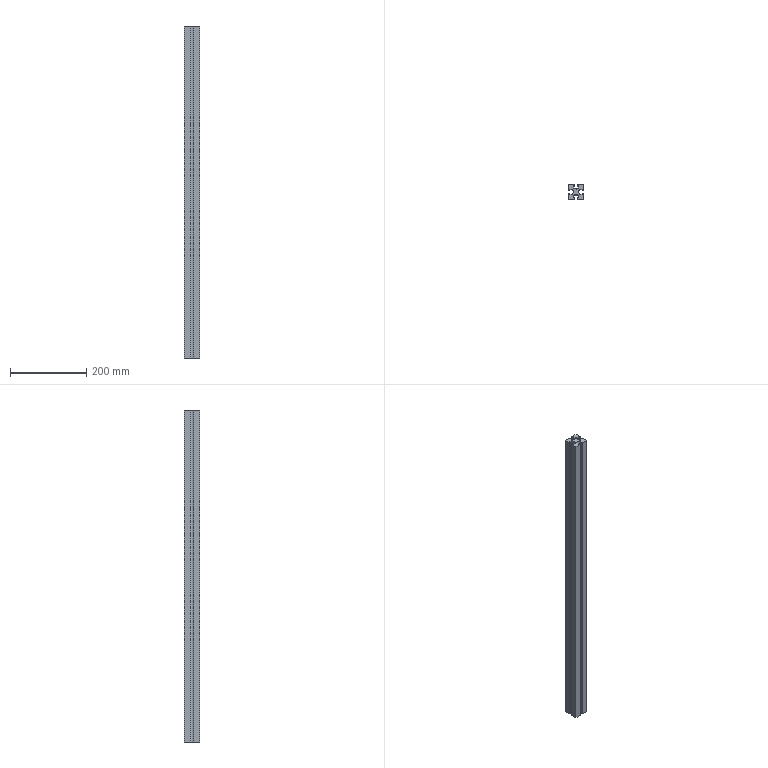Part | NX | 1 solid | 38 faces | box 40 x 40 x 871 mm | volume 871352 mm3 | plane 34 | cylinder 4 | commonest cylinder face diameters 19.333 x2 19.4 x2
STEP:
#1=CARTESIAN_POINT('',(-125.,655.75,0.));
#2=VERTEX_POINT('',#1);
#3=CARTESIAN_POINT('',(-121.5,655.75,0.));
#4=VERTEX_POINT('',#3);
#5=CARTESIAN_POINT('',(-125.,655.75,0.));
#6=DIRECTION('',(1.,0.,0.));
#7=VECTOR('',#6,1000.);
#8=LINE('',#5,#7);
#9=EDGE_CURVE('',#2,#4,#8,.T.);
#10=ORIENTED_EDGE('',*,*,#9,.T.);
#11=CARTESIAN_POINT('',(-121.5,655.75,-871.));
#12=VERTEX_POINT('',#11);
#13=CARTESIAN_POINT('',(-121.5,655.75,-871.));
#14=DIRECTION('',(0.,0.,1.));
#15=VECTOR('',#14,1000.);
#16=LINE('',#13,#15);
#17=EDGE_CURVE('',#12,#4,#16,.T.);
#18=ORIENTED_EDGE('',*,*,#17,.F.);
#19=CARTESIAN_POINT('',(-125.,655.75,-871.));
#20=VERTEX_POINT('',#19);
#21=CARTESIAN_POINT('',(-125.,655.75,-871.));
#22=DIRECTION('',(1.,0.,0.));
#23=VECTOR('',#22,1000.);
#24=LINE('',#21,#23);
#25=EDGE_CURVE('',#20,#12,#24,.T.);
#26=ORIENTED_EDGE('',*,*,#25,.F.);
#27=CARTESIAN_POINT('',(-125.,655.75,-871.));
#28=DIRECTION('',(0.,0.,1.));
#29=VECTOR('',#28,1000.);
#30=LINE('',#27,#29);
#31=EDGE_CURVE('',#20,#2,#30,.T.);
#32=ORIENTED_EDGE('',*,*,#31,.T.);
#33=EDGE_LOOP('',(#10,#18,#26,#32));
#34=FACE_BOUND('',#33,.T.);
#35=CARTESIAN_POINT('',(-125.,655.75,-871.));
#36=DIRECTION('',(0.,-1.,0.));
#37=DIRECTION('',(0.,0.,-1.));
#38=AXIS2_PLACEMENT_3D('',#35,#36,#37);
#39=PLANE('',#38);
#40=ADVANCED_FACE('',(#34),#39,.F.);
#41=CARTESIAN_POINT('',(-121.5,653.,0.));
#42=VERTEX_POINT('',#41);
#43=CARTESIAN_POINT('',(-121.5,655.75,0.));
#44=DIRECTION('',(0.,-1.,0.));
#45=VECTOR('',#44,1000.);
#46=LINE('',#43,#45);
#47=EDGE_CURVE('',#4,#42,#46,.T.);
#48=ORIENTED_EDGE('',*,*,#47,.T.);
#49=CARTESIAN_POINT('',(-121.5,653.,-871.));
#50=VERTEX_POINT('',#49);
#51=CARTESIAN_POINT('',(-121.5,653.,-871.));
#52=DIRECTION('',(0.,0.,1.));
#53=VECTOR('',#52,1000.);
#54=LINE('',#51,#53);
#55=EDGE_CURVE('',#50,#42,#54,.T.);
#56=ORIENTED_EDGE('',*,*,#55,.F.);
#57=CARTESIAN_POINT('',(-121.5,655.75,-871.));
#58=DIRECTION('',(0.,-1.,0.));
#59=VECTOR('',#58,1000.);
#60=LINE('',#57,#59);
#61=EDGE_CURVE('',#12,#50,#60,.T.);
#62=ORIENTED_EDGE('',*,*,#61,.F.);
#63=ORIENTED_EDGE('',*,*,#17,.T.);
#64=EDGE_LOOP('',(#48,#56,#62,#63));
#65=FACE_BOUND('',#64,.T.);
#66=CARTESIAN_POINT('',(-121.5,655.75,-871.));
#67=DIRECTION('',(-1.,0.,0.));
#68=DIRECTION('',(0.,0.,1.));
#69=AXIS2_PLACEMENT_3D('',#66,#67,#68);
#70=PLANE('',#69);
#71=ADVANCED_FACE('',(#65),#70,.F.);
#72=CARTESIAN_POINT('',(-114.5,653.,0.));
#73=VERTEX_POINT('',#72);
#74=CARTESIAN_POINT('',(-121.5,653.,0.));
#75=DIRECTION('',(1.,0.,0.));
#76=VECTOR('',#75,1000.);
#77=LINE('',#74,#76);
#78=EDGE_CURVE('',#42,#73,#77,.T.);
#79=ORIENTED_EDGE('',*,*,#78,.T.);
#80=CARTESIAN_POINT('',(-114.5,653.,-871.));
#81=VERTEX_POINT('',#80);
#82=CARTESIAN_POINT('',(-114.5,653.,-871.));
#83=DIRECTION('',(0.,0.,1.));
#84=VECTOR('',#83,1000.);
#85=LINE('',#82,#84);
#86=EDGE_CURVE('',#81,#73,#85,.T.);
#87=ORIENTED_EDGE('',*,*,#86,.F.);
#88=CARTESIAN_POINT('',(-121.5,653.,-871.));
#89=DIRECTION('',(1.,0.,0.));
#90=VECTOR('',#89,1000.);
#91=LINE('',#88,#90);
#92=EDGE_CURVE('',#50,#81,#91,.T.);
#93=ORIENTED_EDGE('',*,*,#92,.F.);
#94=ORIENTED_EDGE('',*,*,#55,.T.);
#95=EDGE_LOOP('',(#79,#87,#93,#94));
#96=FACE_BOUND('',#95,.T.);
#97=CARTESIAN_POINT('',(-121.5,653.,-871.));
#98=DIRECTION('',(0.,-1.,0.));
#99=DIRECTION('',(0.,0.,-1.));
#100=AXIS2_PLACEMENT_3D('',#97,#98,#99);
#101=PLANE('',#100);
#102=ADVANCED_FACE('',(#96),#101,.F.);
#103=CARTESIAN_POINT('',(-114.5,667.,0.));
#104=VERTEX_POINT('',#103);
#105=CARTESIAN_POINT('',(-121.167,660.,0.));
#106=DIRECTION('',(0.,0.,1.));
#107=DIRECTION('',(-1.,0.,0.));
#108=AXIS2_PLACEMENT_3D('',#105,#106,#107);
#109=CIRCLE('',#108,9.667);
#110=EDGE_CURVE('',#73,#104,#109,.T.);
#111=ORIENTED_EDGE('',*,*,#110,.T.);
#112=CARTESIAN_POINT('',(-114.5,667.,-871.));
#113=VERTEX_POINT('',#112);
#114=CARTESIAN_POINT('',(-114.5,667.,-871.));
#115=DIRECTION('',(0.,0.,1.));
#116=VECTOR('',#115,1000.);
#117=LINE('',#114,#116);
#118=EDGE_CURVE('',#113,#104,#117,.T.);
#119=ORIENTED_EDGE('',*,*,#118,.F.);
#120=CARTESIAN_POINT('',(-121.167,660.,-871.));
#121=DIRECTION('',(0.,0.,1.));
#122=DIRECTION('',(-1.,0.,0.));
#123=AXIS2_PLACEMENT_3D('',#120,#121,#122);
#124=CIRCLE('',#123,9.667);
#125=EDGE_CURVE('',#81,#113,#124,.T.);
#126=ORIENTED_EDGE('',*,*,#125,.F.);
#127=ORIENTED_EDGE('',*,*,#86,.T.);
#128=EDGE_LOOP('',(#111,#119,#126,#127));
#129=FACE_BOUND('',#128,.T.);
#130=CARTESIAN_POINT('',(-121.167,660.,-871.));
#131=DIRECTION('',(0.,0.,1.));
#132=DIRECTION('',(1.,0.,0.));
#133=AXIS2_PLACEMENT_3D('',#130,#131,#132);
#134=CYLINDRICAL_SURFACE('',#133,9.667);
#135=ADVANCED_FACE('',(#129),#134,.F.);
#136=CARTESIAN_POINT('',(-121.5,667.,0.));
#137=VERTEX_POINT('',#136);
#138=CARTESIAN_POINT('',(-114.5,667.,0.));
#139=DIRECTION('',(-1.,0.,0.));
#140=VECTOR('',#139,1000.);
#141=LINE('',#138,#140);
#142=EDGE_CURVE('',#104,#137,#141,.T.);
#143=ORIENTED_EDGE('',*,*,#142,.T.);
#144=CARTESIAN_POINT('',(-121.5,667.,-871.));
#145=VERTEX_POINT('',#144);
#146=CARTESIAN_POINT('',(-121.5,667.,-871.));
#147=DIRECTION('',(0.,0.,1.));
#148=VECTOR('',#147,1000.);
#149=LINE('',#146,#148);
#150=EDGE_CURVE('',#145,#137,#149,.T.);
#151=ORIENTED_EDGE('',*,*,#150,.F.);
#152=CARTESIAN_POINT('',(-114.5,667.,-871.));
#153=DIRECTION('',(-1.,0.,0.));
#154=VECTOR('',#153,1000.);
#155=LINE('',#152,#154);
#156=EDGE_CURVE('',#113,#145,#155,.T.);
#157=ORIENTED_EDGE('',*,*,#156,.F.);
#158=ORIENTED_EDGE('',*,*,#118,.T.);
#159=EDGE_LOOP('',(#143,#151,#157,#158));
#160=FACE_BOUND('',#159,.T.);
#161=CARTESIAN_POINT('',(-114.5,667.,-871.));
#162=DIRECTION('',(0.,1.,0.));
#163=DIRECTION('',(0.,0.,1.));
#164=AXIS2_PLACEMENT_3D('',#161,#162,#163);
#165=PLANE('',#164);
#166=ADVANCED_FACE('',(#160),#165,.F.);
#167=CARTESIAN_POINT('',(-121.5,664.25,0.));
#168=VERTEX_POINT('',#167);
#169=CARTESIAN_POINT('',(-121.5,667.,0.));
#170=DIRECTION('',(0.,-1.,0.));
#171=VECTOR('',#170,1000.);
#172=LINE('',#169,#171);
#173=EDGE_CURVE('',#137,#168,#172,.T.);
#174=ORIENTED_EDGE('',*,*,#173,.T.);
#175=CARTESIAN_POINT('',(-121.5,664.25,-871.));
#176=VERTEX_POINT('',#175);
#177=CARTESIAN_POINT('',(-121.5,664.25,-871.));
#178=DIRECTION('',(0.,0.,1.));
#179=VECTOR('',#178,1000.);
#180=LINE('',#177,#179);
#181=EDGE_CURVE('',#176,#168,#180,.T.);
#182=ORIENTED_EDGE('',*,*,#181,.F.);
#183=CARTESIAN_POINT('',(-121.5,667.,-871.));
#184=DIRECTION('',(0.,-1.,0.));
#185=VECTOR('',#184,1000.);
#186=LINE('',#183,#185);
#187=EDGE_CURVE('',#145,#176,#186,.T.);
#188=ORIENTED_EDGE('',*,*,#187,.F.);
#189=ORIENTED_EDGE('',*,*,#150,.T.);
#190=EDGE_LOOP('',(#174,#182,#188,#189));
#191=FACE_BOUND('',#190,.T.);
#192=CARTESIAN_POINT('',(-121.5,667.,-871.));
#193=DIRECTION('',(-1.,0.,0.));
#194=DIRECTION('',(0.,0.,1.));
#195=AXIS2_PLACEMENT_3D('',#192,#193,#194);
#196=PLANE('',#195);
#197=ADVANCED_FACE('',(#191),#196,.F.);
#198=CARTESIAN_POINT('',(-125.,664.25,0.));
#199=VERTEX_POINT('',#198);
#200=CARTESIAN_POINT('',(-121.5,664.25,0.));
#201=DIRECTION('',(-1.,0.,0.));
#202=VECTOR('',#201,1000.);
#203=LINE('',#200,#202);
#204=EDGE_CURVE('',#168,#199,#203,.T.);
#205=ORIENTED_EDGE('',*,*,#204,.T.);
#206=CARTESIAN_POINT('',(-125.,664.25,-871.));
#207=VERTEX_POINT('',#206);
#208=CARTESIAN_POINT('',(-125.,664.25,-871.));
#209=DIRECTION('',(0.,0.,1.));
#210=VECTOR('',#209,1000.);
#211=LINE('',#208,#210);
#212=EDGE_CURVE('',#207,#199,#211,.T.);
#213=ORIENTED_EDGE('',*,*,#212,.F.);
#214=CARTESIAN_POINT('',(-121.5,664.25,-871.));
#215=DIRECTION('',(-1.,0.,0.));
#216=VECTOR('',#215,1000.);
#217=LINE('',#214,#216);
#218=EDGE_CURVE('',#176,#207,#217,.T.);
#219=ORIENTED_EDGE('',*,*,#218,.F.);
#220=ORIENTED_EDGE('',*,*,#181,.T.);
#221=EDGE_LOOP('',(#205,#213,#219,#220));
#222=FACE_BOUND('',#221,.T.);
#223=CARTESIAN_POINT('',(-121.5,664.25,-871.));
#224=DIRECTION('',(0.,1.,0.));
#225=DIRECTION('',(0.,0.,1.));
#226=AXIS2_PLACEMENT_3D('',#223,#224,#225);
#227=PLANE('',#226);
#228=ADVANCED_FACE('',(#222),#227,.F.);
#229=CARTESIAN_POINT('',(-125.,680.,0.));
#230=VERTEX_POINT('',#229);
#231=CARTESIAN_POINT('',(-125.,680.,0.));
#232=DIRECTION('',(0.,1.,0.));
#233=VECTOR('',#232,1000.);
#234=LINE('',#231,#233);
#235=EDGE_CURVE('',#199,#230,#234,.T.);
#236=ORIENTED_EDGE('',*,*,#235,.T.);
#237=CARTESIAN_POINT('',(-125.,680.,-871.));
#238=VERTEX_POINT('',#237);
#239=CARTESIAN_POINT('',(-125.,680.,-871.));
#240=DIRECTION('',(0.,0.,1.));
#241=VECTOR('',#240,1000.);
#242=LINE('',#239,#241);
#243=EDGE_CURVE('',#238,#230,#242,.T.);
#244=ORIENTED_EDGE('',*,*,#243,.F.);
#245=CARTESIAN_POINT('',(-125.,664.25,-871.));
#246=DIRECTION('',(0.,1.,0.));
#247=VECTOR('',#246,1000.);
#248=LINE('',#245,#247);
#249=EDGE_CURVE('',#207,#238,#248,.T.);
#250=ORIENTED_EDGE('',*,*,#249,.F.);
#251=ORIENTED_EDGE('',*,*,#212,.T.);
#252=EDGE_LOOP('',(#236,#244,#250,#251));
#253=FACE_BOUND('',#252,.T.);
#254=CARTESIAN_POINT('',(-125.,680.,-871.));
#255=DIRECTION('',(1.,0.,0.));
#256=DIRECTION('',(0.,0.,-1.));
#257=AXIS2_PLACEMENT_3D('',#254,#255,#256);
#258=PLANE('',#257);
#259=ADVANCED_FACE('',(#253),#258,.F.);
#260=CARTESIAN_POINT('',(-109.25,680.,0.));
#261=VERTEX_POINT('',#260);
#262=CARTESIAN_POINT('',(-124.5,680.,0.));
#263=DIRECTION('',(1.,0.,0.));
#264=VECTOR('',#263,1000.);
#265=LINE('',#262,#264);
#266=EDGE_CURVE('',#230,#261,#265,.T.);
#267=ORIENTED_EDGE('',*,*,#266,.T.);
#268=CARTESIAN_POINT('',(-109.25,680.,-871.));
#269=VERTEX_POINT('',#268);
#270=CARTESIAN_POINT('',(-109.25,680.,-871.));
#271=DIRECTION('',(0.,0.,1.));
#272=VECTOR('',#271,1000.);
#273=LINE('',#270,#272);
#274=EDGE_CURVE('',#269,#261,#273,.T.);
#275=ORIENTED_EDGE('',*,*,#274,.F.);
#276=CARTESIAN_POINT('',(-124.5,680.,-871.));
#277=DIRECTION('',(1.,0.,0.));
#278=VECTOR('',#277,1000.);
#279=LINE('',#276,#278);
#280=EDGE_CURVE('',#238,#269,#279,.T.);
#281=ORIENTED_EDGE('',*,*,#280,.F.);
#282=ORIENTED_EDGE('',*,*,#243,.T.);
#283=EDGE_LOOP('',(#267,#275,#281,#282));
#284=FACE_BOUND('',#283,.T.);
#285=CARTESIAN_POINT('',(-124.5,680.,-871.));
#286=DIRECTION('',(0.,-1.,0.));
#287=DIRECTION('',(0.,0.,-1.));
#288=AXIS2_PLACEMENT_3D('',#285,#286,#287);
#289=PLANE('',#288);
#290=ADVANCED_FACE('',(#284),#289,.F.);
#291=CARTESIAN_POINT('',(-109.25,676.5,0.));
#292=VERTEX_POINT('',#291);
#293=CARTESIAN_POINT('',(-109.25,680.,0.));
#294=DIRECTION('',(0.,-1.,0.));
#295=VECTOR('',#294,1000.);
#296=LINE('',#293,#295);
#297=EDGE_CURVE('',#261,#292,#296,.T.);
#298=ORIENTED_EDGE('',*,*,#297,.T.);
#299=CARTESIAN_POINT('',(-109.25,676.5,-871.));
#300=VERTEX_POINT('',#299);
#301=CARTESIAN_POINT('',(-109.25,676.5,-871.));
#302=DIRECTION('',(0.,0.,1.));
#303=VECTOR('',#302,1000.);
#304=LINE('',#301,#303);
#305=EDGE_CURVE('',#300,#292,#304,.T.);
#306=ORIENTED_EDGE('',*,*,#305,.F.);
#307=CARTESIAN_POINT('',(-109.25,680.,-871.));
#308=DIRECTION('',(0.,-1.,0.));
#309=VECTOR('',#308,1000.);
#310=LINE('',#307,#309);
#311=EDGE_CURVE('',#269,#300,#310,.T.);
#312=ORIENTED_EDGE('',*,*,#311,.F.);
#313=ORIENTED_EDGE('',*,*,#274,.T.);
#314=EDGE_LOOP('',(#298,#306,#312,#313));
#315=FACE_BOUND('',#314,.T.);
#316=CARTESIAN_POINT('',(-109.25,680.,-871.));
#317=DIRECTION('',(-1.,0.,0.));
#318=DIRECTION('',(0.,0.,1.));
#319=AXIS2_PLACEMENT_3D('',#316,#317,#318);
#320=PLANE('',#319);
#321=ADVANCED_FACE('',(#315),#320,.F.);
#322=CARTESIAN_POINT('',(-111.5,676.5,0.));
#323=VERTEX_POINT('',#322);
#324=CARTESIAN_POINT('',(-109.25,676.5,0.));
#325=DIRECTION('',(-1.,0.,0.));
#326=VECTOR('',#325,1000.);
#327=LINE('',#324,#326);
#328=EDGE_CURVE('',#292,#323,#327,.T.);
#329=ORIENTED_EDGE('',*,*,#328,.T.);
#330=CARTESIAN_POINT('',(-111.5,676.5,-871.));
#331=VERTEX_POINT('',#330);
#332=CARTESIAN_POINT('',(-111.5,676.5,-871.));
#333=DIRECTION('',(0.,0.,1.));
#334=VECTOR('',#333,1000.);
#335=LINE('',#332,#334);
#336=EDGE_CURVE('',#331,#323,#335,.T.);
#337=ORIENTED_EDGE('',*,*,#336,.F.);
#338=CARTESIAN_POINT('',(-109.25,676.5,-871.));
#339=DIRECTION('',(-1.,0.,0.));
#340=VECTOR('',#339,1000.);
#341=LINE('',#338,#340);
#342=EDGE_CURVE('',#300,#331,#341,.T.);
#343=ORIENTED_EDGE('',*,*,#342,.F.);
#344=ORIENTED_EDGE('',*,*,#305,.T.);
#345=EDGE_LOOP('',(#329,#337,#343,#344));
#346=FACE_BOUND('',#345,.T.);
#347=CARTESIAN_POINT('',(-109.25,676.5,-871.));
#348=DIRECTION('',(0.,1.,0.));
#349=DIRECTION('',(0.,0.,1.));
#350=AXIS2_PLACEMENT_3D('',#347,#348,#349);
#351=PLANE('',#350);
#352=ADVANCED_FACE('',(#346),#351,.F.);
#353=CARTESIAN_POINT('',(-111.5,669.5,0.));
#354=VERTEX_POINT('',#353);
#355=CARTESIAN_POINT('',(-111.5,676.5,0.));
#356=DIRECTION('',(0.,-1.,0.));
#357=VECTOR('',#356,1000.);
#358=LINE('',#355,#357);
#359=EDGE_CURVE('',#323,#354,#358,.T.);
#360=ORIENTED_EDGE('',*,*,#359,.T.);
#361=CARTESIAN_POINT('',(-111.5,669.5,-871.));
#362=VERTEX_POINT('',#361);
#363=CARTESIAN_POINT('',(-111.5,669.5,-871.));
#364=DIRECTION('',(0.,0.,1.));
#365=VECTOR('',#364,1000.);
#366=LINE('',#363,#365);
#367=EDGE_CURVE('',#362,#354,#366,.T.);
#368=ORIENTED_EDGE('',*,*,#367,.F.);
#369=CARTESIAN_POINT('',(-111.5,676.5,-871.));
#370=DIRECTION('',(0.,-1.,0.));
#371=VECTOR('',#370,1000.);
#372=LINE('',#369,#371);
#373=EDGE_CURVE('',#331,#362,#372,.T.);
#374=ORIENTED_EDGE('',*,*,#373,.F.);
#375=ORIENTED_EDGE('',*,*,#336,.T.);
#376=EDGE_LOOP('',(#360,#368,#374,#375));
#377=FACE_BOUND('',#376,.T.);
#378=CARTESIAN_POINT('',(-111.5,676.5,-871.));
#379=DIRECTION('',(-1.,0.,0.));
#380=DIRECTION('',(0.,0.,1.));
#381=AXIS2_PLACEMENT_3D('',#378,#379,#380);
#382=PLANE('',#381);
#383=ADVANCED_FACE('',(#377),#382,.F.);
#384=CARTESIAN_POINT('',(-98.5,669.5,0.));
#385=VERTEX_POINT('',#384);
#386=CARTESIAN_POINT('',(-105.,676.7,0.));
#387=DIRECTION('',(0.,0.,1.));
#388=DIRECTION('',(-1.,0.,0.));
#389=AXIS2_PLACEMENT_3D('',#386,#387,#388);
#390=CIRCLE('',#389,9.7);
#391=EDGE_CURVE('',#354,#385,#390,.T.);
#392=ORIENTED_EDGE('',*,*,#391,.T.);
#393=CARTESIAN_POINT('',(-98.5,669.5,-871.));
#394=VERTEX_POINT('',#393);
#395=CARTESIAN_POINT('',(-98.5,669.5,-871.));
#396=DIRECTION('',(0.,0.,1.));
#397=VECTOR('',#396,1000.);
#398=LINE('',#395,#397);
#399=EDGE_CURVE('',#394,#385,#398,.T.);
#400=ORIENTED_EDGE('',*,*,#399,.F.);
#401=CARTESIAN_POINT('',(-105.,676.7,-871.));
#402=DIRECTION('',(0.,0.,1.));
#403=DIRECTION('',(-1.,0.,0.));
#404=AXIS2_PLACEMENT_3D('',#401,#402,#403);
#405=CIRCLE('',#404,9.7);
#406=EDGE_CURVE('',#362,#394,#405,.T.);
#407=ORIENTED_EDGE('',*,*,#406,.F.);
#408=ORIENTED_EDGE('',*,*,#367,.T.);
#409=EDGE_LOOP('',(#392,#400,#407,#408));
#410=FACE_BOUND('',#409,.T.);
#411=CARTESIAN_POINT('',(-105.,676.7,-871.));
#412=DIRECTION('',(0.,0.,1.));
#413=DIRECTION('',(1.,0.,0.));
#414=AXIS2_PLACEMENT_3D('',#411,#412,#413);
#415=CYLINDRICAL_SURFACE('',#414,9.7);
#416=ADVANCED_FACE('',(#410),#415,.F.);
#417=CARTESIAN_POINT('',(-98.5,676.5,0.));
#418=VERTEX_POINT('',#417);
#419=CARTESIAN_POINT('',(-98.5,669.5,0.));
#420=DIRECTION('',(0.,1.,0.));
#421=VECTOR('',#420,1000.);
#422=LINE('',#419,#421);
#423=EDGE_CURVE('',#385,#418,#422,.T.);
#424=ORIENTED_EDGE('',*,*,#423,.T.);
#425=CARTESIAN_POINT('',(-98.5,676.5,-871.));
#426=VERTEX_POINT('',#425);
#427=CARTESIAN_POINT('',(-98.5,676.5,-871.));
#428=DIRECTION('',(0.,0.,1.));
#429=VECTOR('',#428,1000.);
#430=LINE('',#427,#429);
#431=EDGE_CURVE('',#426,#418,#430,.T.);
#432=ORIENTED_EDGE('',*,*,#431,.F.);
#433=CARTESIAN_POINT('',(-98.5,669.5,-871.));
#434=DIRECTION('',(0.,1.,0.));
#435=VECTOR('',#434,1000.);
#436=LINE('',#433,#435);
#437=EDGE_CURVE('',#394,#426,#436,.T.);
#438=ORIENTED_EDGE('',*,*,#437,.F.);
#439=ORIENTED_EDGE('',*,*,#399,.T.);
#440=EDGE_LOOP('',(#424,#432,#438,#439));
#441=FACE_BOUND('',#440,.T.);
#442=CARTESIAN_POINT('',(-98.5,669.5,-871.));
#443=DIRECTION('',(1.,0.,0.));
#444=DIRECTION('',(0.,0.,-1.));
#445=AXIS2_PLACEMENT_3D('',#442,#443,#444);
#446=PLANE('',#445);
#447=ADVANCED_FACE('',(#441),#446,.F.);
#448=CARTESIAN_POINT('',(-100.75,676.5,0.));
#449=VERTEX_POINT('',#448);
#450=CARTESIAN_POINT('',(-98.5,676.5,0.));
#451=DIRECTION('',(-1.,0.,0.));
#452=VECTOR('',#451,1000.);
#453=LINE('',#450,#452);
#454=EDGE_CURVE('',#418,#449,#453,.T.);
#455=ORIENTED_EDGE('',*,*,#454,.T.);
#456=CARTESIAN_POINT('',(-100.75,676.5,-871.));
#457=VERTEX_POINT('',#456);
#458=CARTESIAN_POINT('',(-100.75,676.5,-871.));
#459=DIRECTION('',(0.,0.,1.));
#460=VECTOR('',#459,1000.);
#461=LINE('',#458,#460);
#462=EDGE_CURVE('',#457,#449,#461,.T.);
#463=ORIENTED_EDGE('',*,*,#462,.F.);
#464=CARTESIAN_POINT('',(-98.5,676.5,-871.));
#465=DIRECTION('',(-1.,0.,0.));
#466=VECTOR('',#465,1000.);
#467=LINE('',#464,#466);
#468=EDGE_CURVE('',#426,#457,#467,.T.);
#469=ORIENTED_EDGE('',*,*,#468,.F.);
#470=ORIENTED_EDGE('',*,*,#431,.T.);
#471=EDGE_LOOP('',(#455,#463,#469,#470));
#472=FACE_BOUND('',#471,.T.);
#473=CARTESIAN_POINT('',(-98.5,676.5,-871.));
#474=DIRECTION('',(0.,1.,0.));
#475=DIRECTION('',(0.,0.,1.));
#476=AXIS2_PLACEMENT_3D('',#473,#474,#475);
#477=PLANE('',#476);
#478=ADVANCED_FACE('',(#472),#477,.F.);
#479=CARTESIAN_POINT('',(-100.75,680.,0.));
#480=VERTEX_POINT('',#479);
#481=CARTESIAN_POINT('',(-100.75,676.5,0.));
#482=DIRECTION('',(0.,1.,0.));
#483=VECTOR('',#482,1000.);
#484=LINE('',#481,#483);
#485=EDGE_CURVE('',#449,#480,#484,.T.);
#486=ORIENTED_EDGE('',*,*,#485,.T.);
#487=CARTESIAN_POINT('',(-100.75,680.,-871.));
#488=VERTEX_POINT('',#487);
#489=CARTESIAN_POINT('',(-100.75,680.,-871.));
#490=DIRECTION('',(0.,0.,1.));
#491=VECTOR('',#490,1000.);
#492=LINE('',#489,#491);
#493=EDGE_CURVE('',#488,#480,#492,.T.);
#494=ORIENTED_EDGE('',*,*,#493,.F.);
#495=CARTESIAN_POINT('',(-100.75,676.5,-871.));
#496=DIRECTION('',(0.,1.,0.));
#497=VECTOR('',#496,1000.);
#498=LINE('',#495,#497);
#499=EDGE_CURVE('',#457,#488,#498,.T.);
#500=ORIENTED_EDGE('',*,*,#499,.F.);
#501=ORIENTED_EDGE('',*,*,#462,.T.);
#502=EDGE_LOOP('',(#486,#494,#500,#501));
#503=FACE_BOUND('',#502,.T.);
#504=CARTESIAN_POINT('',(-100.75,676.5,-871.));
#505=DIRECTION('',(1.,0.,0.));
#506=DIRECTION('',(0.,0.,-1.));
#507=AXIS2_PLACEMENT_3D('',#504,#505,#506);
#508=PLANE('',#507);
#509=ADVANCED_FACE('',(#503),#508,.F.);
#510=CARTESIAN_POINT('',(-85.,680.,0.));
#511=VERTEX_POINT('',#510);
#512=CARTESIAN_POINT('',(-85.5,680.,0.));
#513=DIRECTION('',(1.,0.,0.));
#514=VECTOR('',#513,1000.);
#515=LINE('',#512,#514);
#516=EDGE_CURVE('',#480,#511,#515,.T.);
#517=ORIENTED_EDGE('',*,*,#516,.T.);
#518=CARTESIAN_POINT('',(-85.,680.,-871.));
#519=VERTEX_POINT('',#518);
#520=CARTESIAN_POINT('',(-85.,680.,-871.));
#521=DIRECTION('',(0.,0.,1.));
#522=VECTOR('',#521,1000.);
#523=LINE('',#520,#522);
#524=EDGE_CURVE('',#519,#511,#523,.T.);
#525=ORIENTED_EDGE('',*,*,#524,.F.);
#526=CARTESIAN_POINT('',(-100.75,680.,-871.));
#527=DIRECTION('',(1.,0.,0.));
#528=VECTOR('',#527,1000.);
#529=LINE('',#526,#528);
#530=EDGE_CURVE('',#488,#519,#529,.T.);
#531=ORIENTED_EDGE('',*,*,#530,.F.);
#532=ORIENTED_EDGE('',*,*,#493,.T.);
#533=EDGE_LOOP('',(#517,#525,#531,#532));
#534=FACE_BOUND('',#533,.T.);
#535=CARTESIAN_POINT('',(-85.5,680.,-871.));
#536=DIRECTION('',(0.,-1.,0.));
#537=DIRECTION('',(0.,0.,-1.));
#538=AXIS2_PLACEMENT_3D('',#535,#536,#537);
#539=PLANE('',#538);
#540=ADVANCED_FACE('',(#534),#539,.F.);
#541=CARTESIAN_POINT('',(-85.,664.25,0.));
#542=VERTEX_POINT('',#541);
#543=CARTESIAN_POINT('',(-85.,679.5,0.));
#544=DIRECTION('',(0.,-1.,0.));
#545=VECTOR('',#544,1000.);
#546=LINE('',#543,#545);
#547=EDGE_CURVE('',#511,#542,#546,.T.);
#548=ORIENTED_EDGE('',*,*,#547,.T.);
#549=CARTESIAN_POINT('',(-85.,664.25,-871.));
#550=VERTEX_POINT('',#549);
#551=CARTESIAN_POINT('',(-85.,664.25,-871.));
#552=DIRECTION('',(0.,0.,1.));
#553=VECTOR('',#552,1000.);
#554=LINE('',#551,#553);
#555=EDGE_CURVE('',#550,#542,#554,.T.);
#556=ORIENTED_EDGE('',*,*,#555,.F.);
#557=CARTESIAN_POINT('',(-85.,680.,-871.));
#558=DIRECTION('',(0.,-1.,0.));
#559=VECTOR('',#558,1000.);
#560=LINE('',#557,#559);
#561=EDGE_CURVE('',#519,#550,#560,.T.);
#562=ORIENTED_EDGE('',*,*,#561,.F.);
#563=ORIENTED_EDGE('',*,*,#524,.T.);
#564=EDGE_LOOP('',(#548,#556,#562,#563));
#565=FACE_BOUND('',#564,.T.);
#566=CARTESIAN_POINT('',(-85.,679.5,-871.));
#567=DIRECTION('',(-1.,0.,0.));
#568=DIRECTION('',(0.,0.,1.));
#569=AXIS2_PLACEMENT_3D('',#566,#567,#568);
#570=PLANE('',#569);
#571=ADVANCED_FACE('',(#565),#570,.F.);
#572=CARTESIAN_POINT('',(-88.5,664.25,0.));
#573=VERTEX_POINT('',#572);
#574=CARTESIAN_POINT('',(-85.,664.25,0.));
#575=DIRECTION('',(-1.,0.,0.));
#576=VECTOR('',#575,1000.);
#577=LINE('',#574,#576);
#578=EDGE_CURVE('',#542,#573,#577,.T.);
#579=ORIENTED_EDGE('',*,*,#578,.T.);
#580=CARTESIAN_POINT('',(-88.5,664.25,-871.));
#581=VERTEX_POINT('',#580);
#582=CARTESIAN_POINT('',(-88.5,664.25,-871.));
#583=DIRECTION('',(0.,0.,1.));
#584=VECTOR('',#583,1000.);
#585=LINE('',#582,#584);
#586=EDGE_CURVE('',#581,#573,#585,.T.);
#587=ORIENTED_EDGE('',*,*,#586,.F.);
#588=CARTESIAN_POINT('',(-85.,664.25,-871.));
#589=DIRECTION('',(-1.,0.,0.));
#590=VECTOR('',#589,1000.);
#591=LINE('',#588,#590);
#592=EDGE_CURVE('',#550,#581,#591,.T.);
#593=ORIENTED_EDGE('',*,*,#592,.F.);
#594=ORIENTED_EDGE('',*,*,#555,.T.);
#595=EDGE_LOOP('',(#579,#587,#593,#594));
#596=FACE_BOUND('',#595,.T.);
#597=CARTESIAN_POINT('',(-85.,664.25,-871.));
#598=DIRECTION('',(0.,1.,0.));
#599=DIRECTION('',(0.,0.,1.));
#600=AXIS2_PLACEMENT_3D('',#597,#598,#599);
#601=PLANE('',#600);
#602=ADVANCED_FACE('',(#596),#601,.F.);
#603=CARTESIAN_POINT('',(-88.5,667.,0.));
#604=VERTEX_POINT('',#603);
#605=CARTESIAN_POINT('',(-88.5,664.25,0.));
#606=DIRECTION('',(0.,1.,0.));
#607=VECTOR('',#606,1000.);
#608=LINE('',#605,#607);
#609=EDGE_CURVE('',#573,#604,#608,.T.);
#610=ORIENTED_EDGE('',*,*,#609,.T.);
#611=CARTESIAN_POINT('',(-88.5,667.,-871.));
#612=VERTEX_POINT('',#611);
#613=CARTESIAN_POINT('',(-88.5,667.,-871.));
#614=DIRECTION('',(0.,0.,1.));
#615=VECTOR('',#614,1000.);
#616=LINE('',#613,#615);
#617=EDGE_CURVE('',#612,#604,#616,.T.);
#618=ORIENTED_EDGE('',*,*,#617,.F.);
#619=CARTESIAN_POINT('',(-88.5,664.25,-871.));
#620=DIRECTION('',(0.,1.,0.));
#621=VECTOR('',#620,1000.);
#622=LINE('',#619,#621);
#623=EDGE_CURVE('',#581,#612,#622,.T.);
#624=ORIENTED_EDGE('',*,*,#623,.F.);
#625=ORIENTED_EDGE('',*,*,#586,.T.);
#626=EDGE_LOOP('',(#610,#618,#624,#625));
#627=FACE_BOUND('',#626,.T.);
#628=CARTESIAN_POINT('',(-88.5,664.25,-871.));
#629=DIRECTION('',(1.,0.,0.));
#630=DIRECTION('',(0.,0.,-1.));
#631=AXIS2_PLACEMENT_3D('',#628,#629,#630);
#632=PLANE('',#631);
#633=ADVANCED_FACE('',(#627),#632,.F.);
#634=CARTESIAN_POINT('',(-95.5,667.,0.));
#635=VERTEX_POINT('',#634);
#636=CARTESIAN_POINT('',(-88.5,667.,0.));
#637=DIRECTION('',(-1.,0.,0.));
#638=VECTOR('',#637,1000.);
#639=LINE('',#636,#638);
#640=EDGE_CURVE('',#604,#635,#639,.T.);
#641=ORIENTED_EDGE('',*,*,#640,.T.);
#642=CARTESIAN_POINT('',(-95.5,667.,-871.));
#643=VERTEX_POINT('',#642);
#644=CARTESIAN_POINT('',(-95.5,667.,-871.));
#645=DIRECTION('',(0.,0.,1.));
#646=VECTOR('',#645,1000.);
#647=LINE('',#644,#646);
#648=EDGE_CURVE('',#643,#635,#647,.T.);
#649=ORIENTED_EDGE('',*,*,#648,.F.);
#650=CARTESIAN_POINT('',(-88.5,667.,-871.));
#651=DIRECTION('',(-1.,0.,0.));
#652=VECTOR('',#651,1000.);
#653=LINE('',#650,#652);
#654=EDGE_CURVE('',#612,#643,#653,.T.);
#655=ORIENTED_EDGE('',*,*,#654,.F.);
#656=ORIENTED_EDGE('',*,*,#617,.T.);
#657=EDGE_LOOP('',(#641,#649,#655,#656));
#658=FACE_BOUND('',#657,.T.);
#659=CARTESIAN_POINT('',(-88.5,667.,-871.));
#660=DIRECTION('',(0.,1.,0.));
#661=DIRECTION('',(0.,0.,1.));
#662=AXIS2_PLACEMENT_3D('',#659,#660,#661);
#663=PLANE('',#662);
#664=ADVANCED_FACE('',(#658),#663,.F.);
#665=CARTESIAN_POINT('',(-95.5,653.,0.));
#666=VERTEX_POINT('',#665);
#667=CARTESIAN_POINT('',(-88.833,660.,0.));
#668=DIRECTION('',(0.,0.,1.));
#669=DIRECTION('',(-1.,0.,0.));
#670=AXIS2_PLACEMENT_3D('',#667,#668,#669);
#671=CIRCLE('',#670,9.667);
#672=EDGE_CURVE('',#635,#666,#671,.T.);
#673=ORIENTED_EDGE('',*,*,#672,.T.);
#674=CARTESIAN_POINT('',(-95.5,653.,-871.));
#675=VERTEX_POINT('',#674);
#676=CARTESIAN_POINT('',(-95.5,653.,-871.));
#677=DIRECTION('',(0.,0.,1.));
#678=VECTOR('',#677,1000.);
#679=LINE('',#676,#678);
#680=EDGE_CURVE('',#675,#666,#679,.T.);
#681=ORIENTED_EDGE('',*,*,#680,.F.);
#682=CARTESIAN_POINT('',(-88.833,660.,-871.));
#683=DIRECTION('',(0.,0.,1.));
#684=DIRECTION('',(-1.,0.,0.));
#685=AXIS2_PLACEMENT_3D('',#682,#683,#684);
#686=CIRCLE('',#685,9.667);
#687=EDGE_CURVE('',#643,#675,#686,.T.);
#688=ORIENTED_EDGE('',*,*,#687,.F.);
#689=ORIENTED_EDGE('',*,*,#648,.T.);
#690=EDGE_LOOP('',(#673,#681,#688,#689));
#691=FACE_BOUND('',#690,.T.);
#692=CARTESIAN_POINT('',(-88.833,660.,-871.));
#693=DIRECTION('',(0.,0.,1.));
#694=DIRECTION('',(1.,0.,0.));
#695=AXIS2_PLACEMENT_3D('',#692,#693,#694);
#696=CYLINDRICAL_SURFACE('',#695,9.667);
#697=ADVANCED_FACE('',(#691),#696,.F.);
#698=CARTESIAN_POINT('',(-88.5,653.,0.));
#699=VERTEX_POINT('',#698);
#700=CARTESIAN_POINT('',(-95.5,653.,0.));
#701=DIRECTION('',(1.,0.,0.));
#702=VECTOR('',#701,1000.);
#703=LINE('',#700,#702);
#704=EDGE_CURVE('',#666,#699,#703,.T.);
#705=ORIENTED_EDGE('',*,*,#704,.T.);
#706=CARTESIAN_POINT('',(-88.5,653.,-871.));
#707=VERTEX_POINT('',#706);
#708=CARTESIAN_POINT('',(-88.5,653.,-871.));
#709=DIRECTION('',(0.,0.,1.));
#710=VECTOR('',#709,1000.);
#711=LINE('',#708,#710);
#712=EDGE_CURVE('',#707,#699,#711,.T.);
#713=ORIENTED_EDGE('',*,*,#712,.F.);
#714=CARTESIAN_POINT('',(-95.5,653.,-871.));
#715=DIRECTION('',(1.,0.,0.));
#716=VECTOR('',#715,1000.);
#717=LINE('',#714,#716);
#718=EDGE_CURVE('',#675,#707,#717,.T.);
#719=ORIENTED_EDGE('',*,*,#718,.F.);
#720=ORIENTED_EDGE('',*,*,#680,.T.);
#721=EDGE_LOOP('',(#705,#713,#719,#720));
#722=FACE_BOUND('',#721,.T.);
#723=CARTESIAN_POINT('',(-95.5,653.,-871.));
#724=DIRECTION('',(0.,-1.,0.));
#725=DIRECTION('',(0.,0.,-1.));
#726=AXIS2_PLACEMENT_3D('',#723,#724,#725);
#727=PLANE('',#726);
#728=ADVANCED_FACE('',(#722),#727,.F.);
#729=CARTESIAN_POINT('',(-88.5,655.75,0.));
#730=VERTEX_POINT('',#729);
#731=CARTESIAN_POINT('',(-88.5,653.,0.));
#732=DIRECTION('',(0.,1.,0.));
#733=VECTOR('',#732,1000.);
#734=LINE('',#731,#733);
#735=EDGE_CURVE('',#699,#730,#734,.T.);
#736=ORIENTED_EDGE('',*,*,#735,.T.);
#737=CARTESIAN_POINT('',(-88.5,655.75,-871.));
#738=VERTEX_POINT('',#737);
#739=CARTESIAN_POINT('',(-88.5,655.75,-871.));
#740=DIRECTION('',(0.,0.,1.));
#741=VECTOR('',#740,1000.);
#742=LINE('',#739,#741);
#743=EDGE_CURVE('',#738,#730,#742,.T.);
#744=ORIENTED_EDGE('',*,*,#743,.F.);
#745=CARTESIAN_POINT('',(-88.5,653.,-871.));
#746=DIRECTION('',(0.,1.,0.));
#747=VECTOR('',#746,1000.);
#748=LINE('',#745,#747);
#749=EDGE_CURVE('',#707,#738,#748,.T.);
#750=ORIENTED_EDGE('',*,*,#749,.F.);
#751=ORIENTED_EDGE('',*,*,#712,.T.);
#752=EDGE_LOOP('',(#736,#744,#750,#751));
#753=FACE_BOUND('',#752,.T.);
#754=CARTESIAN_POINT('',(-88.5,653.,-871.));
#755=DIRECTION('',(1.,0.,0.));
#756=DIRECTION('',(0.,0.,-1.));
#757=AXIS2_PLACEMENT_3D('',#754,#755,#756);
#758=PLANE('',#757);
#759=ADVANCED_FACE('',(#753),#758,.F.);
#760=CARTESIAN_POINT('',(-85.,655.75,0.));
#761=VERTEX_POINT('',#760);
#762=CARTESIAN_POINT('',(-88.5,655.75,0.));
#763=DIRECTION('',(1.,0.,0.));
#764=VECTOR('',#763,1000.);
#765=LINE('',#762,#764);
#766=EDGE_CURVE('',#730,#761,#765,.T.);
#767=ORIENTED_EDGE('',*,*,#766,.T.);
#768=CARTESIAN_POINT('',(-85.,655.75,-871.));
#769=VERTEX_POINT('',#768);
#770=CARTESIAN_POINT('',(-85.,655.75,-871.));
#771=DIRECTION('',(0.,0.,1.));
#772=VECTOR('',#771,1000.);
#773=LINE('',#770,#772);
#774=EDGE_CURVE('',#769,#761,#773,.T.);
#775=ORIENTED_EDGE('',*,*,#774,.F.);
#776=CARTESIAN_POINT('',(-88.5,655.75,-871.));
#777=DIRECTION('',(1.,0.,0.));
#778=VECTOR('',#777,1000.);
#779=LINE('',#776,#778);
#780=EDGE_CURVE('',#738,#769,#779,.T.);
#781=ORIENTED_EDGE('',*,*,#780,.F.);
#782=ORIENTED_EDGE('',*,*,#743,.T.);
#783=EDGE_LOOP('',(#767,#775,#781,#782));
#784=FACE_BOUND('',#783,.T.);
#785=CARTESIAN_POINT('',(-88.5,655.75,-871.));
#786=DIRECTION('',(0.,-1.,0.));
#787=DIRECTION('',(0.,0.,-1.));
#788=AXIS2_PLACEMENT_3D('',#785,#786,#787);
#789=PLANE('',#788);
#790=ADVANCED_FACE('',(#784),#789,.F.);
#791=CARTESIAN_POINT('',(-85.,640.,0.));
#792=VERTEX_POINT('',#791);
#793=CARTESIAN_POINT('',(-85.,640.5,0.));
#794=DIRECTION('',(0.,-1.,0.));
#795=VECTOR('',#794,1000.);
#796=LINE('',#793,#795);
#797=EDGE_CURVE('',#761,#792,#796,.T.);
#798=ORIENTED_EDGE('',*,*,#797,.T.);
#799=CARTESIAN_POINT('',(-85.,640.,-871.));
#800=VERTEX_POINT('',#799);
#801=CARTESIAN_POINT('',(-85.,640.,-871.));
#802=DIRECTION('',(0.,0.,1.));
#803=VECTOR('',#802,1000.);
#804=LINE('',#801,#803);
#805=EDGE_CURVE('',#800,#792,#804,.T.);
#806=ORIENTED_EDGE('',*,*,#805,.F.);
#807=CARTESIAN_POINT('',(-85.,655.75,-871.));
#808=DIRECTION('',(0.,-1.,0.));
#809=VECTOR('',#808,1000.);
#810=LINE('',#807,#809);
#811=EDGE_CURVE('',#769,#800,#810,.T.);
#812=ORIENTED_EDGE('',*,*,#811,.F.);
#813=ORIENTED_EDGE('',*,*,#774,.T.);
#814=EDGE_LOOP('',(#798,#806,#812,#813));
#815=FACE_BOUND('',#814,.T.);
#816=CARTESIAN_POINT('',(-85.,640.5,-871.));
#817=DIRECTION('',(-1.,0.,0.));
#818=DIRECTION('',(0.,0.,1.));
#819=AXIS2_PLACEMENT_3D('',#816,#817,#818);
#820=PLANE('',#819);
#821=ADVANCED_FACE('',(#815),#820,.F.);
#822=CARTESIAN_POINT('',(-100.75,640.,0.));
#823=VERTEX_POINT('',#822);
#824=CARTESIAN_POINT('',(-85.5,640.,0.));
#825=DIRECTION('',(-1.,0.,0.));
#826=VECTOR('',#825,1000.);
#827=LINE('',#824,#826);
#828=EDGE_CURVE('',#792,#823,#827,.T.);
#829=ORIENTED_EDGE('',*,*,#828,.T.);
#830=CARTESIAN_POINT('',(-100.75,640.,-871.));
#831=VERTEX_POINT('',#830);
#832=CARTESIAN_POINT('',(-100.75,640.,-871.));
#833=DIRECTION('',(0.,0.,1.));
#834=VECTOR('',#833,1000.);
#835=LINE('',#832,#834);
#836=EDGE_CURVE('',#831,#823,#835,.T.);
#837=ORIENTED_EDGE('',*,*,#836,.F.);
#838=CARTESIAN_POINT('',(-85.,640.,-871.));
#839=DIRECTION('',(-1.,0.,0.));
#840=VECTOR('',#839,1000.);
#841=LINE('',#838,#840);
#842=EDGE_CURVE('',#800,#831,#841,.T.);
#843=ORIENTED_EDGE('',*,*,#842,.F.);
#844=ORIENTED_EDGE('',*,*,#805,.T.);
#845=EDGE_LOOP('',(#829,#837,#843,#844));
#846=FACE_BOUND('',#845,.T.);
#847=CARTESIAN_POINT('',(-85.5,640.,-871.));
#848=DIRECTION('',(0.,1.,0.));
#849=DIRECTION('',(-1.,0.,0.));
#850=AXIS2_PLACEMENT_3D('',#847,#848,#849);
#851=PLANE('',#850);
#852=ADVANCED_FACE('',(#846),#851,.F.);
#853=CARTESIAN_POINT('',(-100.75,643.5,0.));
#854=VERTEX_POINT('',#853);
#855=CARTESIAN_POINT('',(-100.75,640.,0.));
#856=DIRECTION('',(0.,1.,0.));
#857=VECTOR('',#856,1000.);
#858=LINE('',#855,#857);
#859=EDGE_CURVE('',#823,#854,#858,.T.);
#860=ORIENTED_EDGE('',*,*,#859,.T.);
#861=CARTESIAN_POINT('',(-100.75,643.5,-871.));
#862=VERTEX_POINT('',#861);
#863=CARTESIAN_POINT('',(-100.75,643.5,-871.));
#864=DIRECTION('',(0.,0.,1.));
#865=VECTOR('',#864,1000.);
#866=LINE('',#863,#865);
#867=EDGE_CURVE('',#862,#854,#866,.T.);
#868=ORIENTED_EDGE('',*,*,#867,.F.);
#869=CARTESIAN_POINT('',(-100.75,640.,-871.));
#870=DIRECTION('',(0.,1.,0.));
#871=VECTOR('',#870,1000.);
#872=LINE('',#869,#871);
#873=EDGE_CURVE('',#831,#862,#872,.T.);
#874=ORIENTED_EDGE('',*,*,#873,.F.);
#875=ORIENTED_EDGE('',*,*,#836,.T.);
#876=EDGE_LOOP('',(#860,#868,#874,#875));
#877=FACE_BOUND('',#876,.T.);
#878=CARTESIAN_POINT('',(-100.75,640.,-871.));
#879=DIRECTION('',(1.,0.,0.));
#880=DIRECTION('',(0.,0.,-1.));
#881=AXIS2_PLACEMENT_3D('',#878,#879,#880);
#882=PLANE('',#881);
#883=ADVANCED_FACE('',(#877),#882,.F.);
#884=CARTESIAN_POINT('',(-98.5,643.5,0.));
#885=VERTEX_POINT('',#884);
#886=CARTESIAN_POINT('',(-100.75,643.5,0.));
#887=DIRECTION('',(1.,0.,0.));
#888=VECTOR('',#887,1000.);
#889=LINE('',#886,#888);
#890=EDGE_CURVE('',#854,#885,#889,.T.);
#891=ORIENTED_EDGE('',*,*,#890,.T.);
#892=CARTESIAN_POINT('',(-98.5,643.5,-871.));
#893=VERTEX_POINT('',#892);
#894=CARTESIAN_POINT('',(-98.5,643.5,-871.));
#895=DIRECTION('',(0.,0.,1.));
#896=VECTOR('',#895,1000.);
#897=LINE('',#894,#896);
#898=EDGE_CURVE('',#893,#885,#897,.T.);
#899=ORIENTED_EDGE('',*,*,#898,.F.);
#900=CARTESIAN_POINT('',(-100.75,643.5,-871.));
#901=DIRECTION('',(1.,0.,0.));
#902=VECTOR('',#901,1000.);
#903=LINE('',#900,#902);
#904=EDGE_CURVE('',#862,#893,#903,.T.);
#905=ORIENTED_EDGE('',*,*,#904,.F.);
#906=ORIENTED_EDGE('',*,*,#867,.T.);
#907=EDGE_LOOP('',(#891,#899,#905,#906));
#908=FACE_BOUND('',#907,.T.);
#909=CARTESIAN_POINT('',(-100.75,643.5,-871.));
#910=DIRECTION('',(0.,-1.,0.));
#911=DIRECTION('',(0.,0.,-1.));
#912=AXIS2_PLACEMENT_3D('',#909,#910,#911);
#913=PLANE('',#912);
#914=ADVANCED_FACE('',(#908),#913,.F.);
#915=CARTESIAN_POINT('',(-98.5,650.5,0.));
#916=VERTEX_POINT('',#915);
#917=CARTESIAN_POINT('',(-98.5,643.5,0.));
#918=DIRECTION('',(0.,1.,0.));
#919=VECTOR('',#918,1000.);
#920=LINE('',#917,#919);
#921=EDGE_CURVE('',#885,#916,#920,.T.);
#922=ORIENTED_EDGE('',*,*,#921,.T.);
#923=CARTESIAN_POINT('',(-98.5,650.5,-871.));
#924=VERTEX_POINT('',#923);
#925=CARTESIAN_POINT('',(-98.5,650.5,-871.));
#926=DIRECTION('',(0.,0.,1.));
#927=VECTOR('',#926,1000.);
#928=LINE('',#925,#927);
#929=EDGE_CURVE('',#924,#916,#928,.T.);
#930=ORIENTED_EDGE('',*,*,#929,.F.);
#931=CARTESIAN_POINT('',(-98.5,643.5,-871.));
#932=DIRECTION('',(0.,1.,0.));
#933=VECTOR('',#932,1000.);
#934=LINE('',#931,#933);
#935=EDGE_CURVE('',#893,#924,#934,.T.);
#936=ORIENTED_EDGE('',*,*,#935,.F.);
#937=ORIENTED_EDGE('',*,*,#898,.T.);
#938=EDGE_LOOP('',(#922,#930,#936,#937));
#939=FACE_BOUND('',#938,.T.);
#940=CARTESIAN_POINT('',(-98.5,643.5,-871.));
#941=DIRECTION('',(1.,0.,0.));
#942=DIRECTION('',(0.,1.,0.));
#943=AXIS2_PLACEMENT_3D('',#940,#941,#942);
#944=PLANE('',#943);
#945=ADVANCED_FACE('',(#939),#944,.F.);
#946=CARTESIAN_POINT('',(-111.5,650.5,0.));
#947=VERTEX_POINT('',#946);
#948=CARTESIAN_POINT('',(-105.,643.3,0.));
#949=DIRECTION('',(0.,0.,1.));
#950=DIRECTION('',(-1.,0.,0.));
#951=AXIS2_PLACEMENT_3D('',#948,#949,#950);
#952=CIRCLE('',#951,9.7);
#953=EDGE_CURVE('',#916,#947,#952,.T.);
#954=ORIENTED_EDGE('',*,*,#953,.T.);
#955=CARTESIAN_POINT('',(-111.5,650.5,-871.));
#956=VERTEX_POINT('',#955);
#957=CARTESIAN_POINT('',(-111.5,650.5,-871.));
#958=DIRECTION('',(0.,0.,1.));
#959=VECTOR('',#958,1000.);
#960=LINE('',#957,#959);
#961=EDGE_CURVE('',#956,#947,#960,.T.);
#962=ORIENTED_EDGE('',*,*,#961,.F.);
#963=CARTESIAN_POINT('',(-105.,643.3,-871.));
#964=DIRECTION('',(0.,0.,1.));
#965=DIRECTION('',(-1.,0.,0.));
#966=AXIS2_PLACEMENT_3D('',#963,#964,#965);
#967=CIRCLE('',#966,9.7);
#968=EDGE_CURVE('',#924,#956,#967,.T.);
#969=ORIENTED_EDGE('',*,*,#968,.F.);
#970=ORIENTED_EDGE('',*,*,#929,.T.);
#971=EDGE_LOOP('',(#954,#962,#969,#970));
#972=FACE_BOUND('',#971,.T.);
#973=CARTESIAN_POINT('',(-105.,643.3,-871.));
#974=DIRECTION('',(0.,0.,1.));
#975=DIRECTION('',(1.,0.,0.));
#976=AXIS2_PLACEMENT_3D('',#973,#974,#975);
#977=CYLINDRICAL_SURFACE('',#976,9.7);
#978=ADVANCED_FACE('',(#972),#977,.F.);
#979=CARTESIAN_POINT('',(-111.5,643.5,0.));
#980=VERTEX_POINT('',#979);
#981=CARTESIAN_POINT('',(-111.5,650.5,0.));
#982=DIRECTION('',(0.,-1.,0.));
#983=VECTOR('',#982,1000.);
#984=LINE('',#981,#983);
#985=EDGE_CURVE('',#947,#980,#984,.T.);
#986=ORIENTED_EDGE('',*,*,#985,.T.);
#987=CARTESIAN_POINT('',(-111.5,643.5,-871.));
#988=VERTEX_POINT('',#987);
#989=CARTESIAN_POINT('',(-111.5,643.5,-871.));
#990=DIRECTION('',(0.,0.,1.));
#991=VECTOR('',#990,1000.);
#992=LINE('',#989,#991);
#993=EDGE_CURVE('',#988,#980,#992,.T.);
#994=ORIENTED_EDGE('',*,*,#993,.F.);
#995=CARTESIAN_POINT('',(-111.5,650.5,-871.));
#996=DIRECTION('',(0.,-1.,0.));
#997=VECTOR('',#996,1000.);
#998=LINE('',#995,#997);
#999=EDGE_CURVE('',#956,#988,#998,.T.);
#1000=ORIENTED_EDGE('',*,*,#999,.F.);
#1001=ORIENTED_EDGE('',*,*,#961,.T.);
#1002=EDGE_LOOP('',(#986,#994,#1000,#1001));
#1003=FACE_BOUND('',#1002,.T.);
#1004=CARTESIAN_POINT('',(-111.5,650.5,-871.));
#1005=DIRECTION('',(-1.,0.,0.));
#1006=DIRECTION('',(0.,-1.,0.));
#1007=AXIS2_PLACEMENT_3D('',#1004,#1005,#1006);
#1008=PLANE('',#1007);
#1009=ADVANCED_FACE('',(#1003),#1008,.F.);
#1010=CARTESIAN_POINT('',(-109.25,643.5,0.));
#1011=VERTEX_POINT('',#1010);
#1012=CARTESIAN_POINT('',(-111.5,643.5,0.));
#1013=DIRECTION('',(1.,0.,0.));
#1014=VECTOR('',#1013,1000.);
#1015=LINE('',#1012,#1014);
#1016=EDGE_CURVE('',#980,#1011,#1015,.T.);
#1017=ORIENTED_EDGE('',*,*,#1016,.T.);
#1018=CARTESIAN_POINT('',(-109.25,643.5,-871.));
#1019=VERTEX_POINT('',#1018);
#1020=CARTESIAN_POINT('',(-109.25,643.5,-871.));
#1021=DIRECTION('',(0.,0.,1.));
#1022=VECTOR('',#1021,1000.);
#1023=LINE('',#1020,#1022);
#1024=EDGE_CURVE('',#1019,#1011,#1023,.T.);
#1025=ORIENTED_EDGE('',*,*,#1024,.F.);
#1026=CARTESIAN_POINT('',(-111.5,643.5,-871.));
#1027=DIRECTION('',(1.,0.,0.));
#1028=VECTOR('',#1027,1000.);
#1029=LINE('',#1026,#1028);
#1030=EDGE_CURVE('',#988,#1019,#1029,.T.);
#1031=ORIENTED_EDGE('',*,*,#1030,.F.);
#1032=ORIENTED_EDGE('',*,*,#993,.T.);
#1033=EDGE_LOOP('',(#1017,#1025,#1031,#1032));
#1034=FACE_BOUND('',#1033,.T.);
#1035=CARTESIAN_POINT('',(-111.5,643.5,-871.));
#1036=DIRECTION('',(0.,-1.,0.));
#1037=DIRECTION('',(0.,0.,-1.));
#1038=AXIS2_PLACEMENT_3D('',#1035,#1036,#1037);
#1039=PLANE('',#1038);
#1040=ADVANCED_FACE('',(#1034),#1039,.F.);
#1041=CARTESIAN_POINT('',(-109.25,640.,0.));
#1042=VERTEX_POINT('',#1041);
#1043=CARTESIAN_POINT('',(-109.25,643.5,0.));
#1044=DIRECTION('',(0.,-1.,0.));
#1045=VECTOR('',#1044,1000.);
#1046=LINE('',#1043,#1045);
#1047=EDGE_CURVE('',#1011,#1042,#1046,.T.);
#1048=ORIENTED_EDGE('',*,*,#1047,.T.);
#1049=CARTESIAN_POINT('',(-109.25,640.,-871.));
#1050=VERTEX_POINT('',#1049);
#1051=CARTESIAN_POINT('',(-109.25,640.,-871.));
#1052=DIRECTION('',(0.,0.,1.));
#1053=VECTOR('',#1052,1000.);
#1054=LINE('',#1051,#1053);
#1055=EDGE_CURVE('',#1050,#1042,#1054,.T.);
#1056=ORIENTED_EDGE('',*,*,#1055,.F.);
#1057=CARTESIAN_POINT('',(-109.25,643.5,-871.));
#1058=DIRECTION('',(0.,-1.,0.));
#1059=VECTOR('',#1058,1000.);
#1060=LINE('',#1057,#1059);
#1061=EDGE_CURVE('',#1019,#1050,#1060,.T.);
#1062=ORIENTED_EDGE('',*,*,#1061,.F.);
#1063=ORIENTED_EDGE('',*,*,#1024,.T.);
#1064=EDGE_LOOP('',(#1048,#1056,#1062,#1063));
#1065=FACE_BOUND('',#1064,.T.);
#1066=CARTESIAN_POINT('',(-109.25,643.5,-871.));
#1067=DIRECTION('',(-1.,0.,0.));
#1068=DIRECTION('',(0.,0.,1.));
#1069=AXIS2_PLACEMENT_3D('',#1066,#1067,#1068);
#1070=PLANE('',#1069);
#1071=ADVANCED_FACE('',(#1065),#1070,.F.);
#1072=CARTESIAN_POINT('',(-125.,640.,0.));
#1073=VERTEX_POINT('',#1072);
#1074=CARTESIAN_POINT('',(-125.,640.,0.));
#1075=DIRECTION('',(-1.,0.,0.));
#1076=VECTOR('',#1075,1000.);
#1077=LINE('',#1074,#1076);
#1078=EDGE_CURVE('',#1042,#1073,#1077,.T.);
#1079=ORIENTED_EDGE('',*,*,#1078,.T.);
#1080=CARTESIAN_POINT('',(-125.,640.,-871.));
#1081=VERTEX_POINT('',#1080);
#1082=CARTESIAN_POINT('',(-125.,640.,-871.));
#1083=DIRECTION('',(0.,0.,1.));
#1084=VECTOR('',#1083,1000.);
#1085=LINE('',#1082,#1084);
#1086=EDGE_CURVE('',#1081,#1073,#1085,.T.);
#1087=ORIENTED_EDGE('',*,*,#1086,.F.);
#1088=CARTESIAN_POINT('',(-109.25,640.,-871.));
#1089=DIRECTION('',(-1.,0.,0.));
#1090=VECTOR('',#1089,1000.);
#1091=LINE('',#1088,#1090);
#1092=EDGE_CURVE('',#1050,#1081,#1091,.T.);
#1093=ORIENTED_EDGE('',*,*,#1092,.F.);
#1094=ORIENTED_EDGE('',*,*,#1055,.T.);
#1095=EDGE_LOOP('',(#1079,#1087,#1093,#1094));
#1096=FACE_BOUND('',#1095,.T.);
#1097=CARTESIAN_POINT('',(-125.,640.,-871.));
#1098=DIRECTION('',(0.,1.,0.));
#1099=DIRECTION('',(0.,0.,1.));
#1100=AXIS2_PLACEMENT_3D('',#1097,#1098,#1099);
#1101=PLANE('',#1100);
#1102=ADVANCED_FACE('',(#1096),#1101,.F.);
#1103=CARTESIAN_POINT('',(-125.,640.5,0.));
#1104=DIRECTION('',(0.,1.,0.));
#1105=VECTOR('',#1104,1000.);
#1106=LINE('',#1103,#1105);
#1107=EDGE_CURVE('',#1073,#2,#1106,.T.);
#1108=ORIENTED_EDGE('',*,*,#1107,.T.);
#1109=ORIENTED_EDGE('',*,*,#31,.F.);
#1110=CARTESIAN_POINT('',(-125.,640.5,-871.));
#1111=DIRECTION('',(0.,1.,0.));
#1112=VECTOR('',#1111,1000.);
#1113=LINE('',#1110,#1112);
#1114=EDGE_CURVE('',#1081,#20,#1113,.T.);
#1115=ORIENTED_EDGE('',*,*,#1114,.F.);
#1116=ORIENTED_EDGE('',*,*,#1086,.T.);
#1117=EDGE_LOOP('',(#1108,#1109,#1115,#1116));
#1118=FACE_BOUND('',#1117,.T.);
#1119=CARTESIAN_POINT('',(-125.,640.5,-871.));
#1120=DIRECTION('',(1.,0.,0.));
#1121=DIRECTION('',(0.,0.,-1.));
#1122=AXIS2_PLACEMENT_3D('',#1119,#1120,#1121);
#1123=PLANE('',#1122);
#1124=ADVANCED_FACE('',(#1118),#1123,.F.);
#1125=ORIENTED_EDGE('',*,*,#1114,.T.);
#1126=ORIENTED_EDGE('',*,*,#25,.T.);
#1127=ORIENTED_EDGE('',*,*,#61,.T.);
#1128=ORIENTED_EDGE('',*,*,#92,.T.);
#1129=ORIENTED_EDGE('',*,*,#125,.T.);
#1130=ORIENTED_EDGE('',*,*,#156,.T.);
#1131=ORIENTED_EDGE('',*,*,#187,.T.);
#1132=ORIENTED_EDGE('',*,*,#218,.T.);
#1133=ORIENTED_EDGE('',*,*,#249,.T.);
#1134=ORIENTED_EDGE('',*,*,#280,.T.);
#1135=ORIENTED_EDGE('',*,*,#311,.T.);
#1136=ORIENTED_EDGE('',*,*,#342,.T.);
#1137=ORIENTED_EDGE('',*,*,#373,.T.);
#1138=ORIENTED_EDGE('',*,*,#406,.T.);
#1139=ORIENTED_EDGE('',*,*,#437,.T.);
#1140=ORIENTED_EDGE('',*,*,#468,.T.);
#1141=ORIENTED_EDGE('',*,*,#499,.T.);
#1142=ORIENTED_EDGE('',*,*,#530,.T.);
#1143=ORIENTED_EDGE('',*,*,#561,.T.);
#1144=ORIENTED_EDGE('',*,*,#592,.T.);
#1145=ORIENTED_EDGE('',*,*,#623,.T.);
#1146=ORIENTED_EDGE('',*,*,#654,.T.);
#1147=ORIENTED_EDGE('',*,*,#687,.T.);
#1148=ORIENTED_EDGE('',*,*,#718,.T.);
#1149=ORIENTED_EDGE('',*,*,#749,.T.);
#1150=ORIENTED_EDGE('',*,*,#780,.T.);
#1151=ORIENTED_EDGE('',*,*,#811,.T.);
#1152=ORIENTED_EDGE('',*,*,#842,.T.);
#1153=ORIENTED_EDGE('',*,*,#873,.T.);
#1154=ORIENTED_EDGE('',*,*,#904,.T.);
#1155=ORIENTED_EDGE('',*,*,#935,.T.);
#1156=ORIENTED_EDGE('',*,*,#968,.T.);
#1157=ORIENTED_EDGE('',*,*,#999,.T.);
#1158=ORIENTED_EDGE('',*,*,#1030,.T.);
#1159=ORIENTED_EDGE('',*,*,#1061,.T.);
#1160=ORIENTED_EDGE('',*,*,#1092,.T.);
#1161=EDGE_LOOP('',(#1125,#1126,#1127,#1128,#1129,#1130,#1131,#1132,#1133,#1134,#1135,#1136,#1137,#1138,#1139,#1140,#1141,#1142,#1143,#1144,#1145,#1146,#1147,#1148,#1149,#1150,#1151,#1152,#1153,#1154,#1155,#1156,#1157,#1158,#1159,#1160));
#1162=FACE_BOUND('',#1161,.T.);
#1163=CARTESIAN_POINT('',(-121.167,660.,-871.));
#1164=DIRECTION('',(0.,0.,-1.));
#1165=DIRECTION('',(-1.,0.,0.));
#1166=AXIS2_PLACEMENT_3D('',#1163,#1164,#1165);
#1167=PLANE('',#1166);
#1168=ADVANCED_FACE('',(#1162),#1167,.T.);
#1169=ORIENTED_EDGE('',*,*,#9,.F.);
#1170=ORIENTED_EDGE('',*,*,#1107,.F.);
#1171=ORIENTED_EDGE('',*,*,#1078,.F.);
#1172=ORIENTED_EDGE('',*,*,#1047,.F.);
#1173=ORIENTED_EDGE('',*,*,#1016,.F.);
#1174=ORIENTED_EDGE('',*,*,#985,.F.);
#1175=ORIENTED_EDGE('',*,*,#953,.F.);
#1176=ORIENTED_EDGE('',*,*,#921,.F.);
#1177=ORIENTED_EDGE('',*,*,#890,.F.);
#1178=ORIENTED_EDGE('',*,*,#859,.F.);
#1179=ORIENTED_EDGE('',*,*,#828,.F.);
#1180=ORIENTED_EDGE('',*,*,#797,.F.);
#1181=ORIENTED_EDGE('',*,*,#766,.F.);
#1182=ORIENTED_EDGE('',*,*,#735,.F.);
#1183=ORIENTED_EDGE('',*,*,#704,.F.);
#1184=ORIENTED_EDGE('',*,*,#672,.F.);
#1185=ORIENTED_EDGE('',*,*,#640,.F.);
#1186=ORIENTED_EDGE('',*,*,#609,.F.);
#1187=ORIENTED_EDGE('',*,*,#578,.F.);
#1188=ORIENTED_EDGE('',*,*,#547,.F.);
#1189=ORIENTED_EDGE('',*,*,#516,.F.);
#1190=ORIENTED_EDGE('',*,*,#485,.F.);
#1191=ORIENTED_EDGE('',*,*,#454,.F.);
#1192=ORIENTED_EDGE('',*,*,#423,.F.);
#1193=ORIENTED_EDGE('',*,*,#391,.F.);
#1194=ORIENTED_EDGE('',*,*,#359,.F.);
#1195=ORIENTED_EDGE('',*,*,#328,.F.);
#1196=ORIENTED_EDGE('',*,*,#297,.F.);
#1197=ORIENTED_EDGE('',*,*,#266,.F.);
#1198=ORIENTED_EDGE('',*,*,#235,.F.);
#1199=ORIENTED_EDGE('',*,*,#204,.F.);
#1200=ORIENTED_EDGE('',*,*,#173,.F.);
#1201=ORIENTED_EDGE('',*,*,#142,.F.);
#1202=ORIENTED_EDGE('',*,*,#110,.F.);
#1203=ORIENTED_EDGE('',*,*,#78,.F.);
#1204=ORIENTED_EDGE('',*,*,#47,.F.);
#1205=EDGE_LOOP('',(#1169,#1170,#1171,#1172,#1173,#1174,#1175,#1176,#1177,#1178,#1179,#1180,#1181,#1182,#1183,#1184,#1185,#1186,#1187,#1188,#1189,#1190,#1191,#1192,#1193,#1194,#1195,#1196,#1197,#1198,#1199,#1200,#1201,#1202,#1203,#1204));
#1206=FACE_BOUND('',#1205,.T.);
#1207=CARTESIAN_POINT('',(-121.167,660.,0.));
#1208=DIRECTION('',(0.,0.,-1.));
#1209=DIRECTION('',(-1.,0.,0.));
#1210=AXIS2_PLACEMENT_3D('',#1207,#1208,#1209);
#1211=PLANE('',#1210);
#1212=ADVANCED_FACE('',(#1206),#1211,.F.);
#1213=CLOSED_SHELL('',(#40,#71,#102,#135,#166,#197,#228,#259,#290,#321,#352,#383,#416,#447,#478,#509,#540,#571,#602,#633,#664,#697,#728,#759,#790,#821,#852,#883,#914,#945,#978,#1009,#1040,#1071,#1102,#1124,#1168,#1212));
#1214=MANIFOLD_SOLID_BREP('',#1213);
#1215=(LENGTH_UNIT()NAMED_UNIT(*)SI_UNIT(.MILLI.,.METRE.));
#1216=UNCERTAINTY_MEASURE_WITH_UNIT(LENGTH_MEASURE(0.00001),#1215,'','');
#1217=(NAMED_UNIT(*)PLANE_ANGLE_UNIT()SI_UNIT($,.RADIAN.));
#1218=(NAMED_UNIT(*)SI_UNIT($,.STERADIAN.)SOLID_ANGLE_UNIT());
#1219=(GEOMETRIC_REPRESENTATION_CONTEXT(3)GLOBAL_UNCERTAINTY_ASSIGNED_CONTEXT((#1216))GLOBAL_UNIT_ASSIGNED_CONTEXT((#1215,#1217,#1218))REPRESENTATION_CONTEXT('',''));
#1220=ADVANCED_BREP_SHAPE_REPRESENTATION('',(#1214),#1219);